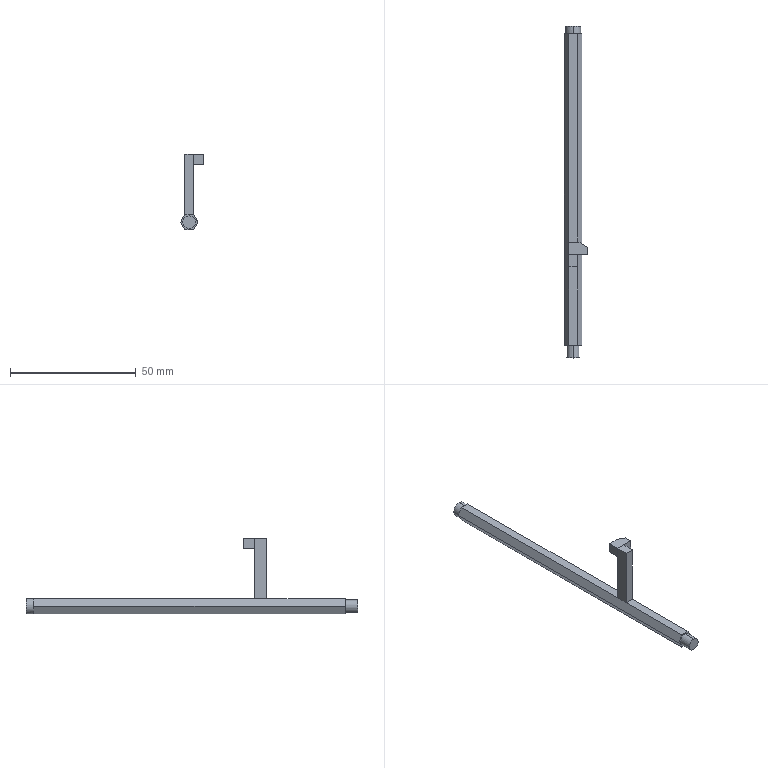Part | SolidWorks | features ICE 6, Cut 3, BaseBody 1, Chamfer 1 | 2 solids | 33 faces | box 9.182 x 132 x 30 mm | volume 4582 mm3 | plane 29 | cylinder 4 | commonest cylinder face diameters 5 x2 6 x2
STEP:
#1=CARTESIAN_POINT('',(-126.829,300.,155.684));
#2=VERTEX_POINT('',#1);
#3=CARTESIAN_POINT('',(-126.829,300.,149.684));
#4=VERTEX_POINT('',#3);
#5=CARTESIAN_POINT('',(-126.829,300.,152.684));
#6=DIRECTION('',(0.,1.,0.));
#7=DIRECTION('',(0.,0.,1.));
#8=AXIS2_PLACEMENT_3D('',#5,#6,#7);
#9=CIRCLE('',#8,3.);
#10=EDGE_CURVE('',#2,#4,#9,.T.);
#11=ORIENTED_EDGE('',*,*,#10,.F.);
#12=CARTESIAN_POINT('',(-126.829,297.,155.684));
#13=VERTEX_POINT('',#12);
#14=CARTESIAN_POINT('',(-126.829,302.,155.684));
#15=DIRECTION('',(0.,-1.,0.));
#16=VECTOR('',#15,1000.);
#17=LINE('',#14,#16);
#18=EDGE_CURVE('',#2,#13,#17,.T.);
#19=ORIENTED_EDGE('',*,*,#18,.T.);
#20=CARTESIAN_POINT('',(-124.231,297.,154.184));
#21=VERTEX_POINT('',#20);
#22=CARTESIAN_POINT('',(-126.829,297.,152.684));
#23=DIRECTION('',(0.,1.,0.));
#24=DIRECTION('',(1.,0.,0.));
#25=AXIS2_PLACEMENT_3D('',#22,#23,#24);
#26=CIRCLE('',#25,3.);
#27=EDGE_CURVE('',#13,#21,#26,.T.);
#28=ORIENTED_EDGE('',*,*,#27,.T.);
#29=CARTESIAN_POINT('',(-124.231,297.,151.184));
#30=VERTEX_POINT('',#29);
#31=CARTESIAN_POINT('',(-126.829,297.,152.684));
#32=DIRECTION('',(0.,1.,0.));
#33=DIRECTION('',(1.,0.,0.));
#34=AXIS2_PLACEMENT_3D('',#31,#32,#33);
#35=CIRCLE('',#34,3.);
#36=EDGE_CURVE('',#21,#30,#35,.T.);
#37=ORIENTED_EDGE('',*,*,#36,.T.);
#38=CARTESIAN_POINT('',(-126.829,297.,149.684));
#39=VERTEX_POINT('',#38);
#40=CARTESIAN_POINT('',(-126.829,297.,152.684));
#41=DIRECTION('',(0.,1.,0.));
#42=DIRECTION('',(1.,0.,0.));
#43=AXIS2_PLACEMENT_3D('',#40,#41,#42);
#44=CIRCLE('',#43,3.);
#45=EDGE_CURVE('',#30,#39,#44,.T.);
#46=ORIENTED_EDGE('',*,*,#45,.T.);
#47=CARTESIAN_POINT('',(-126.829,302.,149.684));
#48=DIRECTION('',(0.,-1.,0.));
#49=VECTOR('',#48,1000.);
#50=LINE('',#47,#49);
#51=EDGE_CURVE('',#4,#39,#50,.T.);
#52=ORIENTED_EDGE('',*,*,#51,.F.);
#53=EDGE_LOOP('',(#11,#19,#28,#37,#46,#52));
#54=FACE_OUTER_BOUND('',#53,.T.);
#55=CARTESIAN_POINT('',(-126.829,302.,152.684));
#56=DIRECTION('',(0.,-1.,0.));
#57=DIRECTION('',(0.,0.,-1.));
#58=AXIS2_PLACEMENT_3D('',#55,#56,#57);
#59=CYLINDRICAL_SURFACE('',#58,3.);
#60=ADVANCED_FACE('',(#54),#59,.T.);
#61=CARTESIAN_POINT('',(-126.829,168.,150.184));
#62=VERTEX_POINT('',#61);
#63=CARTESIAN_POINT('',(-126.829,168.,155.184));
#64=VERTEX_POINT('',#63);
#65=CARTESIAN_POINT('',(-126.829,168.,152.684));
#66=DIRECTION('',(0.,-1.,0.));
#67=DIRECTION('',(1.,0.,0.));
#68=AXIS2_PLACEMENT_3D('',#65,#66,#67);
#69=CIRCLE('',#68,2.5);
#70=EDGE_CURVE('',#62,#64,#69,.T.);
#71=ORIENTED_EDGE('',*,*,#70,.F.);
#72=CARTESIAN_POINT('',(-126.829,173.,150.184));
#73=VERTEX_POINT('',#72);
#74=CARTESIAN_POINT('',(-126.829,168.,150.184));
#75=DIRECTION('',(0.,1.,0.));
#76=VECTOR('',#75,1000.);
#77=LINE('',#74,#76);
#78=EDGE_CURVE('',#62,#73,#77,.T.);
#79=ORIENTED_EDGE('',*,*,#78,.T.);
#80=CARTESIAN_POINT('',(-126.829,173.,155.184));
#81=VERTEX_POINT('',#80);
#82=CARTESIAN_POINT('',(-126.829,173.,152.684));
#83=DIRECTION('',(0.,-1.,0.));
#84=DIRECTION('',(1.,0.,0.));
#85=AXIS2_PLACEMENT_3D('',#82,#83,#84);
#86=CIRCLE('',#85,2.5);
#87=EDGE_CURVE('',#73,#81,#86,.T.);
#88=ORIENTED_EDGE('',*,*,#87,.T.);
#89=CARTESIAN_POINT('',(-126.829,168.,155.184));
#90=DIRECTION('',(0.,1.,0.));
#91=VECTOR('',#90,1000.);
#92=LINE('',#89,#91);
#93=EDGE_CURVE('',#64,#81,#92,.T.);
#94=ORIENTED_EDGE('',*,*,#93,.F.);
#95=EDGE_LOOP('',(#71,#79,#88,#94));
#96=FACE_OUTER_BOUND('',#95,.T.);
#97=CARTESIAN_POINT('',(-126.829,168.,152.684));
#98=DIRECTION('',(0.,1.,0.));
#99=DIRECTION('',(0.,0.,1.));
#100=AXIS2_PLACEMENT_3D('',#97,#98,#99);
#101=CYLINDRICAL_SURFACE('',#100,2.5);
#102=ADVANCED_FACE('',(#96),#101,.T.);
#103=CARTESIAN_POINT('',(-128.561,209.118,179.684));
#104=VERTEX_POINT('',#103);
#105=CARTESIAN_POINT('',(-128.561,204.238,179.684));
#106=VERTEX_POINT('',#105);
#107=CARTESIAN_POINT('',(-128.561,217.498,179.684));
#108=DIRECTION('',(0.,-1.,0.));
#109=VECTOR('',#108,1000.);
#110=LINE('',#107,#109);
#111=EDGE_CURVE('',#104,#106,#110,.T.);
#112=ORIENTED_EDGE('',*,*,#111,.F.);
#113=CARTESIAN_POINT('',(-128.561,209.118,155.684));
#114=VERTEX_POINT('',#113);
#115=CARTESIAN_POINT('',(-128.561,209.118,155.684));
#116=DIRECTION('',(0.,0.,1.));
#117=VECTOR('',#116,1000.);
#118=LINE('',#115,#117);
#119=EDGE_CURVE('',#114,#104,#118,.T.);
#120=ORIENTED_EDGE('',*,*,#119,.F.);
#121=CARTESIAN_POINT('',(-128.561,204.238,155.684));
#122=VERTEX_POINT('',#121);
#123=CARTESIAN_POINT('',(-128.561,306.,155.684));
#124=DIRECTION('',(0.,-1.,0.));
#125=VECTOR('',#124,1000.);
#126=LINE('',#123,#125);
#127=EDGE_CURVE('',#114,#122,#126,.T.);
#128=ORIENTED_EDGE('',*,*,#127,.T.);
#129=CARTESIAN_POINT('',(-128.561,204.238,179.684));
#130=DIRECTION('',(0.,0.,1.));
#131=VECTOR('',#130,1000.);
#132=LINE('',#129,#131);
#133=EDGE_CURVE('',#122,#106,#132,.T.);
#134=ORIENTED_EDGE('',*,*,#133,.T.);
#135=EDGE_LOOP('',(#112,#120,#128,#134));
#136=FACE_OUTER_BOUND('',#135,.T.);
#137=CARTESIAN_POINT('',(-128.561,214.621,195.684));
#138=DIRECTION('',(1.,0.,0.));
#139=DIRECTION('',(0.,0.,-1.));
#140=AXIS2_PLACEMENT_3D('',#137,#138,#139);
#141=PLANE('',#140);
#142=ADVANCED_FACE('',(#136),#141,.F.);
#143=CARTESIAN_POINT('',(-125.096,209.118,179.684));
#144=VERTEX_POINT('',#143);
#145=CARTESIAN_POINT('',(5.,209.118,179.684));
#146=DIRECTION('',(1.,0.,0.));
#147=VECTOR('',#146,1000.);
#148=LINE('',#145,#147);
#149=EDGE_CURVE('',#104,#144,#148,.T.);
#150=ORIENTED_EDGE('',*,*,#149,.F.);
#151=ORIENTED_EDGE('',*,*,#111,.T.);
#152=CARTESIAN_POINT('',(-125.096,204.238,179.684));
#153=VERTEX_POINT('',#152);
#154=CARTESIAN_POINT('',(-125.096,204.238,179.684));
#155=DIRECTION('',(-1.,0.,0.));
#156=VECTOR('',#155,1000.);
#157=LINE('',#154,#156);
#158=EDGE_CURVE('',#153,#106,#157,.T.);
#159=ORIENTED_EDGE('',*,*,#158,.F.);
#160=CARTESIAN_POINT('',(-125.096,207.238,179.684));
#161=DIRECTION('',(0.,1.,0.));
#162=VECTOR('',#161,1000.);
#163=LINE('',#160,#162);
#164=EDGE_CURVE('',#153,#144,#163,.T.);
#165=ORIENTED_EDGE('',*,*,#164,.T.);
#166=EDGE_LOOP('',(#150,#151,#159,#165));
#167=FACE_OUTER_BOUND('',#166,.T.);
#168=CARTESIAN_POINT('',(5.,0.,179.684));
#169=DIRECTION('',(0.,0.,1.));
#170=DIRECTION('',(1.,0.,0.));
#171=AXIS2_PLACEMENT_3D('',#168,#169,#170);
#172=PLANE('',#171);
#173=ADVANCED_FACE('',(#167),#172,.T.);
#174=ORIENTED_EDGE('',*,*,#45,.F.);
#175=CARTESIAN_POINT('',(-125.097,297.,149.684));
#176=VERTEX_POINT('',#175);
#177=CARTESIAN_POINT('',(-123.365,297.,152.684));
#178=DIRECTION('',(-0.5,0.,-0.866));
#179=VECTOR('',#178,1000.);
#180=LINE('',#177,#179);
#181=EDGE_CURVE('',#30,#176,#180,.T.);
#182=ORIENTED_EDGE('',*,*,#181,.T.);
#183=CARTESIAN_POINT('',(-125.097,297.,149.684));
#184=DIRECTION('',(-1.,0.,0.));
#185=VECTOR('',#184,1000.);
#186=LINE('',#183,#185);
#187=EDGE_CURVE('',#176,#39,#186,.T.);
#188=ORIENTED_EDGE('',*,*,#187,.T.);
#189=EDGE_LOOP('',(#174,#182,#188));
#190=FACE_OUTER_BOUND('',#189,.T.);
#191=CARTESIAN_POINT('',(-195.,297.,35.));
#192=DIRECTION('',(0.,1.,0.));
#193=DIRECTION('',(0.,0.,-1.));
#194=AXIS2_PLACEMENT_3D('',#191,#192,#193);
#195=PLANE('',#194);
#196=ADVANCED_FACE('',(#190),#195,.T.);
#197=CARTESIAN_POINT('',(-129.427,297.,151.184));
#198=VERTEX_POINT('',#197);
#199=CARTESIAN_POINT('',(-126.829,297.,152.684));
#200=DIRECTION('',(0.,1.,0.));
#201=DIRECTION('',(1.,0.,0.));
#202=AXIS2_PLACEMENT_3D('',#199,#200,#201);
#203=CIRCLE('',#202,3.);
#204=EDGE_CURVE('',#39,#198,#203,.T.);
#205=ORIENTED_EDGE('',*,*,#204,.F.);
#206=CARTESIAN_POINT('',(-128.561,297.,149.684));
#207=VERTEX_POINT('',#206);
#208=CARTESIAN_POINT('',(-125.097,297.,149.684));
#209=DIRECTION('',(-1.,0.,0.));
#210=VECTOR('',#209,1000.);
#211=LINE('',#208,#210);
#212=EDGE_CURVE('',#39,#207,#211,.T.);
#213=ORIENTED_EDGE('',*,*,#212,.T.);
#214=CARTESIAN_POINT('',(-128.561,297.,149.684));
#215=DIRECTION('',(-0.5,0.,0.866));
#216=VECTOR('',#215,1000.);
#217=LINE('',#214,#216);
#218=EDGE_CURVE('',#207,#198,#217,.T.);
#219=ORIENTED_EDGE('',*,*,#218,.T.);
#220=EDGE_LOOP('',(#205,#213,#219));
#221=FACE_OUTER_BOUND('',#220,.T.);
#222=CARTESIAN_POINT('',(-195.,297.,35.));
#223=DIRECTION('',(0.,1.,0.));
#224=DIRECTION('',(0.,0.,-1.));
#225=AXIS2_PLACEMENT_3D('',#222,#223,#224);
#226=PLANE('',#225);
#227=ADVANCED_FACE('',(#221),#226,.T.);
#228=CARTESIAN_POINT('',(-129.427,297.,154.184));
#229=VERTEX_POINT('',#228);
#230=CARTESIAN_POINT('',(-126.829,297.,152.684));
#231=DIRECTION('',(0.,1.,0.));
#232=DIRECTION('',(1.,0.,0.));
#233=AXIS2_PLACEMENT_3D('',#230,#231,#232);
#234=CIRCLE('',#233,3.);
#235=EDGE_CURVE('',#198,#229,#234,.T.);
#236=ORIENTED_EDGE('',*,*,#235,.F.);
#237=CARTESIAN_POINT('',(-130.293,297.,152.684));
#238=VERTEX_POINT('',#237);
#239=CARTESIAN_POINT('',(-128.561,297.,149.684));
#240=DIRECTION('',(-0.5,0.,0.866));
#241=VECTOR('',#240,1000.);
#242=LINE('',#239,#241);
#243=EDGE_CURVE('',#198,#238,#242,.T.);
#244=ORIENTED_EDGE('',*,*,#243,.T.);
#245=CARTESIAN_POINT('',(-130.293,297.,152.684));
#246=DIRECTION('',(0.5,0.,0.866));
#247=VECTOR('',#246,1000.);
#248=LINE('',#245,#247);
#249=EDGE_CURVE('',#238,#229,#248,.T.);
#250=ORIENTED_EDGE('',*,*,#249,.T.);
#251=EDGE_LOOP('',(#236,#244,#250));
#252=FACE_OUTER_BOUND('',#251,.T.);
#253=CARTESIAN_POINT('',(-195.,297.,35.));
#254=DIRECTION('',(0.,1.,0.));
#255=DIRECTION('',(0.,0.,-1.));
#256=AXIS2_PLACEMENT_3D('',#253,#254,#255);
#257=PLANE('',#256);
#258=ADVANCED_FACE('',(#252),#257,.T.);
#259=CARTESIAN_POINT('',(-126.829,297.,152.684));
#260=DIRECTION('',(0.,1.,0.));
#261=DIRECTION('',(1.,0.,0.));
#262=AXIS2_PLACEMENT_3D('',#259,#260,#261);
#263=CIRCLE('',#262,3.);
#264=EDGE_CURVE('',#229,#13,#263,.T.);
#265=ORIENTED_EDGE('',*,*,#264,.F.);
#266=CARTESIAN_POINT('',(-128.561,297.,155.684));
#267=VERTEX_POINT('',#266);
#268=CARTESIAN_POINT('',(-130.293,297.,152.684));
#269=DIRECTION('',(0.5,0.,0.866));
#270=VECTOR('',#269,1000.);
#271=LINE('',#268,#270);
#272=EDGE_CURVE('',#229,#267,#271,.T.);
#273=ORIENTED_EDGE('',*,*,#272,.T.);
#274=CARTESIAN_POINT('',(-128.561,297.,155.684));
#275=DIRECTION('',(1.,0.,0.));
#276=VECTOR('',#275,1000.);
#277=LINE('',#274,#276);
#278=EDGE_CURVE('',#267,#13,#277,.T.);
#279=ORIENTED_EDGE('',*,*,#278,.T.);
#280=EDGE_LOOP('',(#265,#273,#279));
#281=FACE_OUTER_BOUND('',#280,.T.);
#282=CARTESIAN_POINT('',(-195.,297.,35.));
#283=DIRECTION('',(0.,1.,0.));
#284=DIRECTION('',(0.,0.,-1.));
#285=AXIS2_PLACEMENT_3D('',#282,#283,#284);
#286=PLANE('',#285);
#287=ADVANCED_FACE('',(#281),#286,.T.);
#288=ORIENTED_EDGE('',*,*,#27,.F.);
#289=CARTESIAN_POINT('',(-125.097,297.,155.684));
#290=VERTEX_POINT('',#289);
#291=CARTESIAN_POINT('',(-128.561,297.,155.684));
#292=DIRECTION('',(1.,0.,0.));
#293=VECTOR('',#292,1000.);
#294=LINE('',#291,#293);
#295=EDGE_CURVE('',#13,#290,#294,.T.);
#296=ORIENTED_EDGE('',*,*,#295,.T.);
#297=CARTESIAN_POINT('',(-125.097,297.,155.684));
#298=DIRECTION('',(0.5,0.,-0.866));
#299=VECTOR('',#298,1000.);
#300=LINE('',#297,#299);
#301=EDGE_CURVE('',#290,#21,#300,.T.);
#302=ORIENTED_EDGE('',*,*,#301,.T.);
#303=EDGE_LOOP('',(#288,#296,#302));
#304=FACE_OUTER_BOUND('',#303,.T.);
#305=CARTESIAN_POINT('',(-195.,297.,35.));
#306=DIRECTION('',(0.,1.,0.));
#307=DIRECTION('',(0.,0.,-1.));
#308=AXIS2_PLACEMENT_3D('',#305,#306,#307);
#309=PLANE('',#308);
#310=ADVANCED_FACE('',(#304),#309,.T.);
#311=CARTESIAN_POINT('',(-128.561,214.621,155.684));
#312=DIRECTION('',(0.,-1.,0.));
#313=VECTOR('',#312,1000.);
#314=LINE('',#311,#313);
#315=EDGE_CURVE('',#267,#114,#314,.T.);
#316=ORIENTED_EDGE('',*,*,#315,.T.);
#317=CARTESIAN_POINT('',(-125.096,209.118,155.684));
#318=VERTEX_POINT('',#317);
#319=CARTESIAN_POINT('',(-104.061,209.118,155.684));
#320=DIRECTION('',(-1.,0.,0.));
#321=VECTOR('',#320,1000.);
#322=LINE('',#319,#321);
#323=EDGE_CURVE('',#318,#114,#322,.T.);
#324=ORIENTED_EDGE('',*,*,#323,.F.);
#325=CARTESIAN_POINT('',(-125.096,212.118,155.684));
#326=VERTEX_POINT('',#325);
#327=CARTESIAN_POINT('',(-125.096,0.,155.684));
#328=DIRECTION('',(0.,1.,0.));
#329=VECTOR('',#328,1000.);
#330=LINE('',#327,#329);
#331=EDGE_CURVE('',#318,#326,#330,.T.);
#332=ORIENTED_EDGE('',*,*,#331,.T.);
#333=CARTESIAN_POINT('',(-125.097,212.118,155.684));
#334=VERTEX_POINT('',#333);
#335=CARTESIAN_POINT('',(-115.561,212.118,155.684));
#336=DIRECTION('',(1.,0.,0.));
#337=VECTOR('',#336,1000.);
#338=LINE('',#335,#337);
#339=EDGE_CURVE('',#334,#326,#338,.T.);
#340=ORIENTED_EDGE('',*,*,#339,.F.);
#341=CARTESIAN_POINT('',(-125.097,306.,155.684));
#342=DIRECTION('',(0.,-1.,0.));
#343=VECTOR('',#342,1000.);
#344=LINE('',#341,#343);
#345=EDGE_CURVE('',#290,#334,#344,.T.);
#346=ORIENTED_EDGE('',*,*,#345,.F.);
#347=ORIENTED_EDGE('',*,*,#295,.F.);
#348=ORIENTED_EDGE('',*,*,#278,.F.);
#349=EDGE_LOOP('',(#316,#324,#332,#340,#346,#347,#348));
#350=FACE_OUTER_BOUND('',#349,.T.);
#351=CARTESIAN_POINT('',(-128.561,306.,155.684));
#352=DIRECTION('',(0.,0.,-1.));
#353=DIRECTION('',(-1.,0.,0.));
#354=AXIS2_PLACEMENT_3D('',#351,#352,#353);
#355=PLANE('',#354);
#356=ADVANCED_FACE('',(#350),#355,.F.);
#357=CARTESIAN_POINT('',(-125.097,204.238,155.684));
#358=VERTEX_POINT('',#357);
#359=CARTESIAN_POINT('',(-125.097,173.,155.684));
#360=VERTEX_POINT('',#359);
#361=CARTESIAN_POINT('',(-125.097,306.,155.684));
#362=DIRECTION('',(0.,-1.,0.));
#363=VECTOR('',#362,1000.);
#364=LINE('',#361,#363);
#365=EDGE_CURVE('',#358,#360,#364,.T.);
#366=ORIENTED_EDGE('',*,*,#365,.F.);
#367=CARTESIAN_POINT('',(-125.096,204.238,155.684));
#368=DIRECTION('',(-1.,0.,0.));
#369=VECTOR('',#368,1000.);
#370=LINE('',#367,#369);
#371=EDGE_CURVE('',#358,#122,#370,.T.);
#372=ORIENTED_EDGE('',*,*,#371,.T.);
#373=CARTESIAN_POINT('',(-128.561,173.,155.684));
#374=VERTEX_POINT('',#373);
#375=CARTESIAN_POINT('',(-128.561,306.,155.684));
#376=DIRECTION('',(0.,-1.,0.));
#377=VECTOR('',#376,1000.);
#378=LINE('',#375,#377);
#379=EDGE_CURVE('',#122,#374,#378,.T.);
#380=ORIENTED_EDGE('',*,*,#379,.T.);
#381=CARTESIAN_POINT('',(-128.561,173.,155.684));
#382=DIRECTION('',(1.,0.,0.));
#383=VECTOR('',#382,1000.);
#384=LINE('',#381,#383);
#385=EDGE_CURVE('',#374,#360,#384,.T.);
#386=ORIENTED_EDGE('',*,*,#385,.T.);
#387=EDGE_LOOP('',(#366,#372,#380,#386));
#388=FACE_OUTER_BOUND('',#387,.T.);
#389=CARTESIAN_POINT('',(-128.561,306.,155.684));
#390=DIRECTION('',(0.,0.,-1.));
#391=DIRECTION('',(-1.,0.,0.));
#392=AXIS2_PLACEMENT_3D('',#389,#390,#391);
#393=PLANE('',#392);
#394=ADVANCED_FACE('',(#388),#393,.F.);
#395=ORIENTED_EDGE('',*,*,#345,.T.);
#396=CARTESIAN_POINT('',(-125.096,212.118,155.682));
#397=VERTEX_POINT('',#396);
#398=CARTESIAN_POINT('',(-125.097,212.118,155.684));
#399=DIRECTION('',(0.5,0.,-0.866));
#400=VECTOR('',#399,1000.);
#401=LINE('',#398,#400);
#402=EDGE_CURVE('',#334,#397,#401,.T.);
#403=ORIENTED_EDGE('',*,*,#402,.T.);
#404=CARTESIAN_POINT('',(-125.096,204.238,155.682));
#405=VERTEX_POINT('',#404);
#406=CARTESIAN_POINT('',(-125.096,306.,155.682));
#407=DIRECTION('',(0.,-1.,0.));
#408=VECTOR('',#407,1000.);
#409=LINE('',#406,#408);
#410=EDGE_CURVE('',#397,#405,#409,.T.);
#411=ORIENTED_EDGE('',*,*,#410,.T.);
#412=CARTESIAN_POINT('',(-125.097,204.238,155.684));
#413=DIRECTION('',(-0.5,0.,0.866));
#414=VECTOR('',#413,1000.);
#415=LINE('',#412,#414);
#416=EDGE_CURVE('',#405,#358,#415,.T.);
#417=ORIENTED_EDGE('',*,*,#416,.T.);
#418=ORIENTED_EDGE('',*,*,#365,.T.);
#419=CARTESIAN_POINT('',(-123.365,173.,152.684));
#420=VERTEX_POINT('',#419);
#421=CARTESIAN_POINT('',(-125.097,173.,155.684));
#422=DIRECTION('',(0.5,0.,-0.866));
#423=VECTOR('',#422,1000.);
#424=LINE('',#421,#423);
#425=EDGE_CURVE('',#360,#420,#424,.T.);
#426=ORIENTED_EDGE('',*,*,#425,.T.);
#427=CARTESIAN_POINT('',(-123.365,297.,152.684));
#428=VERTEX_POINT('',#427);
#429=CARTESIAN_POINT('',(-123.365,306.,152.684));
#430=DIRECTION('',(0.,-1.,0.));
#431=VECTOR('',#430,1000.);
#432=LINE('',#429,#431);
#433=EDGE_CURVE('',#428,#420,#432,.T.);
#434=ORIENTED_EDGE('',*,*,#433,.F.);
#435=CARTESIAN_POINT('',(-125.097,297.,155.684));
#436=DIRECTION('',(0.5,0.,-0.866));
#437=VECTOR('',#436,1000.);
#438=LINE('',#435,#437);
#439=EDGE_CURVE('',#21,#428,#438,.T.);
#440=ORIENTED_EDGE('',*,*,#439,.F.);
#441=ORIENTED_EDGE('',*,*,#301,.F.);
#442=EDGE_LOOP('',(#395,#403,#411,#417,#418,#426,#434,#440,#441));
#443=FACE_OUTER_BOUND('',#442,.T.);
#444=CARTESIAN_POINT('',(-125.097,306.,155.684));
#445=DIRECTION('',(-0.866,0.,-0.5));
#446=DIRECTION('',(-0.5,0.,0.866));
#447=AXIS2_PLACEMENT_3D('',#444,#445,#446);
#448=PLANE('',#447);
#449=ADVANCED_FACE('',(#443),#448,.F.);
#450=ORIENTED_EDGE('',*,*,#433,.T.);
#451=CARTESIAN_POINT('',(-125.097,173.,149.684));
#452=VERTEX_POINT('',#451);
#453=CARTESIAN_POINT('',(-123.365,173.,152.684));
#454=DIRECTION('',(-0.5,0.,-0.866));
#455=VECTOR('',#454,1000.);
#456=LINE('',#453,#455);
#457=EDGE_CURVE('',#420,#452,#456,.T.);
#458=ORIENTED_EDGE('',*,*,#457,.T.);
#459=CARTESIAN_POINT('',(-125.097,306.,149.684));
#460=DIRECTION('',(0.,-1.,0.));
#461=VECTOR('',#460,1000.);
#462=LINE('',#459,#461);
#463=EDGE_CURVE('',#176,#452,#462,.T.);
#464=ORIENTED_EDGE('',*,*,#463,.F.);
#465=ORIENTED_EDGE('',*,*,#181,.F.);
#466=CARTESIAN_POINT('',(-123.365,297.,152.684));
#467=DIRECTION('',(-0.5,0.,-0.866));
#468=VECTOR('',#467,1000.);
#469=LINE('',#466,#468);
#470=EDGE_CURVE('',#428,#30,#469,.T.);
#471=ORIENTED_EDGE('',*,*,#470,.F.);
#472=EDGE_LOOP('',(#450,#458,#464,#465,#471));
#473=FACE_OUTER_BOUND('',#472,.T.);
#474=CARTESIAN_POINT('',(-123.365,306.,152.684));
#475=DIRECTION('',(-0.866,0.,0.5));
#476=DIRECTION('',(0.5,0.,0.866));
#477=AXIS2_PLACEMENT_3D('',#474,#475,#476);
#478=PLANE('',#477);
#479=ADVANCED_FACE('',(#473),#478,.F.);
#480=ORIENTED_EDGE('',*,*,#463,.T.);
#481=CARTESIAN_POINT('',(-128.561,173.,149.684));
#482=VERTEX_POINT('',#481);
#483=CARTESIAN_POINT('',(-125.097,173.,149.684));
#484=DIRECTION('',(-1.,0.,0.));
#485=VECTOR('',#484,1000.);
#486=LINE('',#483,#485);
#487=EDGE_CURVE('',#452,#482,#486,.T.);
#488=ORIENTED_EDGE('',*,*,#487,.T.);
#489=CARTESIAN_POINT('',(-128.561,306.,149.684));
#490=DIRECTION('',(0.,-1.,0.));
#491=VECTOR('',#490,1000.);
#492=LINE('',#489,#491);
#493=EDGE_CURVE('',#207,#482,#492,.T.);
#494=ORIENTED_EDGE('',*,*,#493,.F.);
#495=ORIENTED_EDGE('',*,*,#212,.F.);
#496=ORIENTED_EDGE('',*,*,#187,.F.);
#497=EDGE_LOOP('',(#480,#488,#494,#495,#496));
#498=FACE_OUTER_BOUND('',#497,.T.);
#499=CARTESIAN_POINT('',(-125.097,306.,149.684));
#500=DIRECTION('',(0.,0.,1.));
#501=DIRECTION('',(1.,0.,0.));
#502=AXIS2_PLACEMENT_3D('',#499,#500,#501);
#503=PLANE('',#502);
#504=ADVANCED_FACE('',(#498),#503,.F.);
#505=ORIENTED_EDGE('',*,*,#493,.T.);
#506=CARTESIAN_POINT('',(-130.293,173.,152.684));
#507=VERTEX_POINT('',#506);
#508=CARTESIAN_POINT('',(-128.561,173.,149.684));
#509=DIRECTION('',(-0.5,0.,0.866));
#510=VECTOR('',#509,1000.);
#511=LINE('',#508,#510);
#512=EDGE_CURVE('',#482,#507,#511,.T.);
#513=ORIENTED_EDGE('',*,*,#512,.T.);
#514=CARTESIAN_POINT('',(-130.293,306.,152.684));
#515=DIRECTION('',(0.,-1.,0.));
#516=VECTOR('',#515,1000.);
#517=LINE('',#514,#516);
#518=EDGE_CURVE('',#238,#507,#517,.T.);
#519=ORIENTED_EDGE('',*,*,#518,.F.);
#520=ORIENTED_EDGE('',*,*,#243,.F.);
#521=ORIENTED_EDGE('',*,*,#218,.F.);
#522=EDGE_LOOP('',(#505,#513,#519,#520,#521));
#523=FACE_OUTER_BOUND('',#522,.T.);
#524=CARTESIAN_POINT('',(-128.561,306.,149.684));
#525=DIRECTION('',(0.866,0.,0.5));
#526=DIRECTION('',(0.5,0.,-0.866));
#527=AXIS2_PLACEMENT_3D('',#524,#525,#526);
#528=PLANE('',#527);
#529=ADVANCED_FACE('',(#523),#528,.F.);
#530=ORIENTED_EDGE('',*,*,#518,.T.);
#531=CARTESIAN_POINT('',(-130.293,173.,152.684));
#532=DIRECTION('',(0.5,0.,0.866));
#533=VECTOR('',#532,1000.);
#534=LINE('',#531,#533);
#535=EDGE_CURVE('',#507,#374,#534,.T.);
#536=ORIENTED_EDGE('',*,*,#535,.T.);
#537=ORIENTED_EDGE('',*,*,#379,.F.);
#538=ORIENTED_EDGE('',*,*,#127,.F.);
#539=ORIENTED_EDGE('',*,*,#315,.F.);
#540=ORIENTED_EDGE('',*,*,#272,.F.);
#541=ORIENTED_EDGE('',*,*,#249,.F.);
#542=EDGE_LOOP('',(#530,#536,#537,#538,#539,#540,#541));
#543=FACE_OUTER_BOUND('',#542,.T.);
#544=CARTESIAN_POINT('',(-130.293,306.,152.684));
#545=DIRECTION('',(0.866,0.,-0.5));
#546=DIRECTION('',(-0.5,0.,-0.866));
#547=AXIS2_PLACEMENT_3D('',#544,#545,#546);
#548=PLANE('',#547);
#549=ADVANCED_FACE('',(#543),#548,.F.);
#550=ORIENTED_EDGE('',*,*,#36,.F.);
#551=ORIENTED_EDGE('',*,*,#439,.T.);
#552=ORIENTED_EDGE('',*,*,#470,.T.);
#553=EDGE_LOOP('',(#550,#551,#552));
#554=FACE_OUTER_BOUND('',#553,.T.);
#555=CARTESIAN_POINT('',(-195.,297.,35.));
#556=DIRECTION('',(0.,1.,0.));
#557=DIRECTION('',(0.,0.,-1.));
#558=AXIS2_PLACEMENT_3D('',#555,#556,#557);
#559=PLANE('',#558);
#560=ADVANCED_FACE('',(#554),#559,.T.);
#561=CARTESIAN_POINT('',(-126.829,173.,152.684));
#562=DIRECTION('',(0.,-1.,0.));
#563=DIRECTION('',(1.,0.,0.));
#564=AXIS2_PLACEMENT_3D('',#561,#562,#563);
#565=CIRCLE('',#564,2.5);
#566=EDGE_CURVE('',#81,#73,#565,.T.);
#567=ORIENTED_EDGE('',*,*,#566,.F.);
#568=ORIENTED_EDGE('',*,*,#87,.F.);
#569=EDGE_LOOP('',(#567,#568));
#570=FACE_BOUND('',#569,.T.);
#571=ORIENTED_EDGE('',*,*,#385,.F.);
#572=ORIENTED_EDGE('',*,*,#535,.F.);
#573=ORIENTED_EDGE('',*,*,#512,.F.);
#574=ORIENTED_EDGE('',*,*,#487,.F.);
#575=ORIENTED_EDGE('',*,*,#457,.F.);
#576=ORIENTED_EDGE('',*,*,#425,.F.);
#577=EDGE_LOOP('',(#571,#572,#573,#574,#575,#576));
#578=FACE_OUTER_BOUND('',#577,.T.);
#579=CARTESIAN_POINT('',(5.,173.,35.));
#580=DIRECTION('',(0.,1.,0.));
#581=DIRECTION('',(0.,0.,1.));
#582=AXIS2_PLACEMENT_3D('',#579,#580,#581);
#583=PLANE('',#582);
#584=ADVANCED_FACE('',(#570,#578),#583,.F.);
#585=ORIENTED_EDGE('',*,*,#78,.F.);
#586=CARTESIAN_POINT('',(-126.829,168.,152.684));
#587=DIRECTION('',(0.,-1.,0.));
#588=DIRECTION('',(1.,0.,0.));
#589=AXIS2_PLACEMENT_3D('',#586,#587,#588);
#590=CIRCLE('',#589,2.5);
#591=EDGE_CURVE('',#64,#62,#590,.T.);
#592=ORIENTED_EDGE('',*,*,#591,.F.);
#593=ORIENTED_EDGE('',*,*,#93,.T.);
#594=ORIENTED_EDGE('',*,*,#566,.T.);
#595=EDGE_LOOP('',(#585,#592,#593,#594));
#596=FACE_OUTER_BOUND('',#595,.T.);
#597=CARTESIAN_POINT('',(-126.829,168.,152.684));
#598=DIRECTION('',(0.,1.,0.));
#599=DIRECTION('',(0.,0.,1.));
#600=AXIS2_PLACEMENT_3D('',#597,#598,#599);
#601=CYLINDRICAL_SURFACE('',#600,2.5);
#602=ADVANCED_FACE('',(#596),#601,.T.);
#603=ORIENTED_EDGE('',*,*,#591,.T.);
#604=ORIENTED_EDGE('',*,*,#70,.T.);
#605=EDGE_LOOP('',(#603,#604));
#606=FACE_OUTER_BOUND('',#605,.T.);
#607=CARTESIAN_POINT('',(-126.829,168.,152.684));
#608=DIRECTION('',(0.,-1.,0.));
#609=DIRECTION('',(0.,0.,-1.));
#610=AXIS2_PLACEMENT_3D('',#607,#608,#609);
#611=PLANE('',#610);
#612=ADVANCED_FACE('',(#606),#611,.T.);
#613=ORIENTED_EDGE('',*,*,#18,.F.);
#614=CARTESIAN_POINT('',(-126.829,300.,152.684));
#615=DIRECTION('',(0.,1.,0.));
#616=DIRECTION('',(0.,0.,1.));
#617=AXIS2_PLACEMENT_3D('',#614,#615,#616);
#618=CIRCLE('',#617,3.);
#619=EDGE_CURVE('',#4,#2,#618,.T.);
#620=ORIENTED_EDGE('',*,*,#619,.F.);
#621=ORIENTED_EDGE('',*,*,#51,.T.);
#622=ORIENTED_EDGE('',*,*,#204,.T.);
#623=ORIENTED_EDGE('',*,*,#235,.T.);
#624=ORIENTED_EDGE('',*,*,#264,.T.);
#625=EDGE_LOOP('',(#613,#620,#621,#622,#623,#624));
#626=FACE_OUTER_BOUND('',#625,.T.);
#627=CARTESIAN_POINT('',(-126.829,302.,152.684));
#628=DIRECTION('',(0.,-1.,0.));
#629=DIRECTION('',(0.,0.,-1.));
#630=AXIS2_PLACEMENT_3D('',#627,#628,#629);
#631=CYLINDRICAL_SURFACE('',#630,3.);
#632=ADVANCED_FACE('',(#626),#631,.T.);
#633=ORIENTED_EDGE('',*,*,#619,.T.);
#634=ORIENTED_EDGE('',*,*,#10,.T.);
#635=EDGE_LOOP('',(#633,#634));
#636=FACE_OUTER_BOUND('',#635,.T.);
#637=CARTESIAN_POINT('',(-200.,300.,0.));
#638=DIRECTION('',(0.,1.,0.));
#639=DIRECTION('',(0.,0.,-1.));
#640=AXIS2_PLACEMENT_3D('',#637,#638,#639);
#641=PLANE('',#640);
#642=ADVANCED_FACE('',(#636),#641,.T.);
#643=ORIENTED_EDGE('',*,*,#402,.F.);
#644=ORIENTED_EDGE('',*,*,#339,.T.);
#645=CARTESIAN_POINT('',(-125.096,212.118,155.184));
#646=DIRECTION('',(0.,0.,1.));
#647=VECTOR('',#646,1000.);
#648=LINE('',#645,#647);
#649=EDGE_CURVE('',#397,#326,#648,.T.);
#650=ORIENTED_EDGE('',*,*,#649,.F.);
#651=EDGE_LOOP('',(#643,#644,#650));
#652=FACE_OUTER_BOUND('',#651,.T.);
#653=CARTESIAN_POINT('',(-115.561,212.118,173.));
#654=DIRECTION('',(0.,-1.,0.));
#655=DIRECTION('',(0.,0.,-1.));
#656=AXIS2_PLACEMENT_3D('',#653,#654,#655);
#657=PLANE('',#656);
#658=ADVANCED_FACE('',(#652),#657,.F.);
#659=ORIENTED_EDGE('',*,*,#133,.F.);
#660=ORIENTED_EDGE('',*,*,#371,.F.);
#661=ORIENTED_EDGE('',*,*,#416,.F.);
#662=CARTESIAN_POINT('',(-125.096,204.238,179.684));
#663=DIRECTION('',(0.,0.,1.));
#664=VECTOR('',#663,1000.);
#665=LINE('',#662,#664);
#666=EDGE_CURVE('',#405,#153,#665,.T.);
#667=ORIENTED_EDGE('',*,*,#666,.T.);
#668=ORIENTED_EDGE('',*,*,#158,.T.);
#669=EDGE_LOOP('',(#659,#660,#661,#667,#668));
#670=FACE_OUTER_BOUND('',#669,.T.);
#671=CARTESIAN_POINT('',(-125.096,204.238,179.684));
#672=DIRECTION('',(0.,-1.,0.));
#673=DIRECTION('',(0.,0.,-1.));
#674=AXIS2_PLACEMENT_3D('',#671,#672,#673);
#675=PLANE('',#674);
#676=ADVANCED_FACE('',(#670),#675,.T.);
#677=ORIENTED_EDGE('',*,*,#331,.F.);
#678=CARTESIAN_POINT('',(-125.096,209.118,0.));
#679=DIRECTION('',(0.,0.,-1.));
#680=VECTOR('',#679,1000.);
#681=LINE('',#678,#680);
#682=EDGE_CURVE('',#144,#318,#681,.T.);
#683=ORIENTED_EDGE('',*,*,#682,.F.);
#684=ORIENTED_EDGE('',*,*,#164,.F.);
#685=ORIENTED_EDGE('',*,*,#666,.F.);
#686=ORIENTED_EDGE('',*,*,#410,.F.);
#687=ORIENTED_EDGE('',*,*,#649,.T.);
#688=EDGE_LOOP('',(#677,#683,#684,#685,#686,#687));
#689=FACE_OUTER_BOUND('',#688,.T.);
#690=CARTESIAN_POINT('',(-125.096,0.,0.));
#691=DIRECTION('',(1.,0.,0.));
#692=DIRECTION('',(0.,0.,-1.));
#693=AXIS2_PLACEMENT_3D('',#690,#691,#692);
#694=PLANE('',#693);
#695=ADVANCED_FACE('',(#689),#694,.T.);
#696=ORIENTED_EDGE('',*,*,#149,.T.);
#697=ORIENTED_EDGE('',*,*,#682,.T.);
#698=ORIENTED_EDGE('',*,*,#323,.T.);
#699=ORIENTED_EDGE('',*,*,#119,.T.);
#700=EDGE_LOOP('',(#696,#697,#698,#699));
#701=FACE_OUTER_BOUND('',#700,.T.);
#702=CARTESIAN_POINT('',(-104.061,209.118,155.684));
#703=DIRECTION('',(0.,-1.,0.));
#704=DIRECTION('',(0.,0.,-1.));
#705=AXIS2_PLACEMENT_3D('',#702,#703,#704);
#706=PLANE('',#705);
#707=ADVANCED_FACE('',(#701),#706,.F.);
#708=CLOSED_SHELL('',(#60,#102,#142,#173,#196,#227,#258,#287,#310,#356,#394,#449,#479,#504,#529,#549,#560,#584,#602,#612,#632,#642,#658,#676,#695,#707));
#709=MANIFOLD_SOLID_BREP('',#708);
#710=CARTESIAN_POINT('',(-124.111,213.718,175.678));
#711=VERTEX_POINT('',#710);
#712=CARTESIAN_POINT('',(-128.561,213.718,175.678));
#713=VERTEX_POINT('',#712);
#714=CARTESIAN_POINT('',(-128.561,213.718,175.678));
#715=DIRECTION('',(-1.,0.,0.));
#716=VECTOR('',#715,1000.);
#717=LINE('',#714,#716);
#718=EDGE_CURVE('',#711,#713,#717,.T.);
#719=ORIENTED_EDGE('',*,*,#718,.F.);
#720=CARTESIAN_POINT('',(-121.111,211.986,175.678));
#721=VERTEX_POINT('',#720);
#722=CARTESIAN_POINT('',(-122.869,213.001,175.678));
#723=DIRECTION('',(0.866,-0.5,0.));
#724=VECTOR('',#723,1000.);
#725=LINE('',#722,#724);
#726=EDGE_CURVE('',#711,#721,#725,.T.);
#727=ORIENTED_EDGE('',*,*,#726,.T.);
#728=CARTESIAN_POINT('',(-121.111,209.118,175.678));
#729=VERTEX_POINT('',#728);
#730=CARTESIAN_POINT('',(-121.111,211.718,175.678));
#731=DIRECTION('',(0.,1.,0.));
#732=VECTOR('',#731,1000.);
#733=LINE('',#730,#732);
#734=EDGE_CURVE('',#729,#721,#733,.T.);
#735=ORIENTED_EDGE('',*,*,#734,.F.);
#736=CARTESIAN_POINT('',(-128.561,209.118,175.678));
#737=VERTEX_POINT('',#736);
#738=CARTESIAN_POINT('',(-125.111,209.118,175.678));
#739=DIRECTION('',(-1.,0.,0.));
#740=VECTOR('',#739,1000.);
#741=LINE('',#738,#740);
#742=EDGE_CURVE('',#729,#737,#741,.T.);
#743=ORIENTED_EDGE('',*,*,#742,.T.);
#744=CARTESIAN_POINT('',(-128.561,209.118,175.678));
#745=DIRECTION('',(0.,-1.,0.));
#746=VECTOR('',#745,1000.);
#747=LINE('',#744,#746);
#748=EDGE_CURVE('',#713,#737,#747,.T.);
#749=ORIENTED_EDGE('',*,*,#748,.F.);
#750=EDGE_LOOP('',(#719,#727,#735,#743,#749));
#751=FACE_OUTER_BOUND('',#750,.T.);
#752=CARTESIAN_POINT('',(-125.111,209.118,175.678));
#753=DIRECTION('',(0.,0.,-1.));
#754=DIRECTION('',(-1.,0.,0.));
#755=AXIS2_PLACEMENT_3D('',#752,#753,#754);
#756=PLANE('',#755);
#757=ADVANCED_FACE('',(#751),#756,.T.);
#758=CARTESIAN_POINT('',(-121.111,211.986,179.684));
#759=VERTEX_POINT('',#758);
#760=CARTESIAN_POINT('',(-121.111,209.118,179.684));
#761=VERTEX_POINT('',#760);
#762=CARTESIAN_POINT('',(-121.111,211.718,179.684));
#763=DIRECTION('',(0.,-1.,0.));
#764=VECTOR('',#763,1000.);
#765=LINE('',#762,#764);
#766=EDGE_CURVE('',#759,#761,#765,.T.);
#767=ORIENTED_EDGE('',*,*,#766,.F.);
#768=CARTESIAN_POINT('',(-124.111,213.718,179.684));
#769=VERTEX_POINT('',#768);
#770=CARTESIAN_POINT('',(-122.869,213.001,179.684));
#771=DIRECTION('',(-0.866,0.5,0.));
#772=VECTOR('',#771,1000.);
#773=LINE('',#770,#772);
#774=EDGE_CURVE('',#759,#769,#773,.T.);
#775=ORIENTED_EDGE('',*,*,#774,.T.);
#776=CARTESIAN_POINT('',(-128.561,213.718,179.684));
#777=VERTEX_POINT('',#776);
#778=CARTESIAN_POINT('',(-128.561,213.718,179.684));
#779=DIRECTION('',(1.,0.,0.));
#780=VECTOR('',#779,1000.);
#781=LINE('',#778,#780);
#782=EDGE_CURVE('',#777,#769,#781,.T.);
#783=ORIENTED_EDGE('',*,*,#782,.F.);
#784=CARTESIAN_POINT('',(-128.561,209.118,179.684));
#785=VERTEX_POINT('',#784);
#786=CARTESIAN_POINT('',(-128.561,209.118,179.684));
#787=DIRECTION('',(0.,1.,0.));
#788=VECTOR('',#787,1000.);
#789=LINE('',#786,#788);
#790=EDGE_CURVE('',#785,#777,#789,.T.);
#791=ORIENTED_EDGE('',*,*,#790,.F.);
#792=CARTESIAN_POINT('',(-125.111,209.118,179.684));
#793=DIRECTION('',(-1.,0.,0.));
#794=VECTOR('',#793,1000.);
#795=LINE('',#792,#794);
#796=EDGE_CURVE('',#761,#785,#795,.T.);
#797=ORIENTED_EDGE('',*,*,#796,.F.);
#798=EDGE_LOOP('',(#767,#775,#783,#791,#797));
#799=FACE_OUTER_BOUND('',#798,.T.);
#800=CARTESIAN_POINT('',(-125.111,209.118,179.684));
#801=DIRECTION('',(0.,0.,1.));
#802=DIRECTION('',(1.,0.,0.));
#803=AXIS2_PLACEMENT_3D('',#800,#801,#802);
#804=PLANE('',#803);
#805=ADVANCED_FACE('',(#799),#804,.T.);
#806=CARTESIAN_POINT('',(-128.561,209.118,175.678));
#807=DIRECTION('',(0.,0.,1.));
#808=VECTOR('',#807,1000.);
#809=LINE('',#806,#808);
#810=EDGE_CURVE('',#737,#785,#809,.T.);
#811=ORIENTED_EDGE('',*,*,#810,.F.);
#812=ORIENTED_EDGE('',*,*,#742,.F.);
#813=CARTESIAN_POINT('',(-121.111,209.118,179.684));
#814=DIRECTION('',(0.,0.,-1.));
#815=VECTOR('',#814,1000.);
#816=LINE('',#813,#815);
#817=EDGE_CURVE('',#761,#729,#816,.T.);
#818=ORIENTED_EDGE('',*,*,#817,.F.);
#819=ORIENTED_EDGE('',*,*,#796,.T.);
#820=EDGE_LOOP('',(#811,#812,#818,#819));
#821=FACE_OUTER_BOUND('',#820,.T.);
#822=CARTESIAN_POINT('',(-125.111,209.118,175.678));
#823=DIRECTION('',(0.,-1.,0.));
#824=DIRECTION('',(0.,0.,-1.));
#825=AXIS2_PLACEMENT_3D('',#822,#823,#824);
#826=PLANE('',#825);
#827=ADVANCED_FACE('',(#821),#826,.T.);
#828=ORIENTED_EDGE('',*,*,#748,.T.);
#829=ORIENTED_EDGE('',*,*,#810,.T.);
#830=ORIENTED_EDGE('',*,*,#790,.T.);
#831=CARTESIAN_POINT('',(-128.561,213.718,175.678));
#832=DIRECTION('',(0.,0.,1.));
#833=VECTOR('',#832,1000.);
#834=LINE('',#831,#833);
#835=EDGE_CURVE('',#713,#777,#834,.T.);
#836=ORIENTED_EDGE('',*,*,#835,.F.);
#837=EDGE_LOOP('',(#828,#829,#830,#836));
#838=FACE_OUTER_BOUND('',#837,.T.);
#839=CARTESIAN_POINT('',(-128.561,0.,0.));
#840=DIRECTION('',(-1.,0.,0.));
#841=DIRECTION('',(0.,0.,1.));
#842=AXIS2_PLACEMENT_3D('',#839,#840,#841);
#843=PLANE('',#842);
#844=ADVANCED_FACE('',(#838),#843,.T.);
#845=ORIENTED_EDGE('',*,*,#734,.T.);
#846=CARTESIAN_POINT('',(-121.111,211.986,0.));
#847=DIRECTION('',(0.,0.,1.));
#848=VECTOR('',#847,1000.);
#849=LINE('',#846,#848);
#850=EDGE_CURVE('',#721,#759,#849,.T.);
#851=ORIENTED_EDGE('',*,*,#850,.T.);
#852=ORIENTED_EDGE('',*,*,#766,.T.);
#853=ORIENTED_EDGE('',*,*,#817,.T.);
#854=EDGE_LOOP('',(#845,#851,#852,#853));
#855=FACE_OUTER_BOUND('',#854,.T.);
#856=CARTESIAN_POINT('',(-121.111,0.,0.));
#857=DIRECTION('',(1.,0.,0.));
#858=DIRECTION('',(0.,0.,-1.));
#859=AXIS2_PLACEMENT_3D('',#856,#857,#858);
#860=PLANE('',#859);
#861=ADVANCED_FACE('',(#855),#860,.T.);
#862=ORIENTED_EDGE('',*,*,#782,.T.);
#863=CARTESIAN_POINT('',(-124.111,213.718,0.));
#864=DIRECTION('',(0.,0.,-1.));
#865=VECTOR('',#864,1000.);
#866=LINE('',#863,#865);
#867=EDGE_CURVE('',#769,#711,#866,.T.);
#868=ORIENTED_EDGE('',*,*,#867,.T.);
#869=ORIENTED_EDGE('',*,*,#718,.T.);
#870=ORIENTED_EDGE('',*,*,#835,.T.);
#871=EDGE_LOOP('',(#862,#868,#869,#870));
#872=FACE_OUTER_BOUND('',#871,.T.);
#873=CARTESIAN_POINT('',(0.,213.718,0.));
#874=DIRECTION('',(0.,1.,0.));
#875=DIRECTION('',(0.,0.,1.));
#876=AXIS2_PLACEMENT_3D('',#873,#874,#875);
#877=PLANE('',#876);
#878=ADVANCED_FACE('',(#872),#877,.T.);
#879=ORIENTED_EDGE('',*,*,#774,.F.);
#880=ORIENTED_EDGE('',*,*,#850,.F.);
#881=ORIENTED_EDGE('',*,*,#726,.F.);
#882=ORIENTED_EDGE('',*,*,#867,.F.);
#883=EDGE_LOOP('',(#879,#880,#881,#882));
#884=FACE_OUTER_BOUND('',#883,.T.);
#885=CARTESIAN_POINT('',(-124.111,213.718,0.));
#886=DIRECTION('',(-0.5,-0.866,0.));
#887=DIRECTION('',(0.,0.,-1.));
#888=AXIS2_PLACEMENT_3D('',#885,#886,#887);
#889=PLANE('',#888);
#890=ADVANCED_FACE('',(#884),#889,.F.);
#891=CLOSED_SHELL('',(#757,#805,#827,#844,#861,#878,#890));
#892=MANIFOLD_SOLID_BREP('',#891);
#893=CARTESIAN_POINT('',(0.,0.,0.));
#894=DIRECTION('',(0.,0.,1.));
#895=DIRECTION('',(1.,0.,0.));
#896=AXIS2_PLACEMENT_3D('',#893,#894,#895);
#897=(LENGTH_UNIT()NAMED_UNIT(*)SI_UNIT(.MILLI.,.METRE.));
#898=UNCERTAINTY_MEASURE_WITH_UNIT(LENGTH_MEASURE(0.00001),#897,'','');
#899=(NAMED_UNIT(*)PLANE_ANGLE_UNIT()SI_UNIT($,.RADIAN.));
#900=(NAMED_UNIT(*)SI_UNIT($,.STERADIAN.)SOLID_ANGLE_UNIT());
#901=(GEOMETRIC_REPRESENTATION_CONTEXT(3)GLOBAL_UNCERTAINTY_ASSIGNED_CONTEXT((#898))GLOBAL_UNIT_ASSIGNED_CONTEXT((#897,#899,#900))REPRESENTATION_CONTEXT('',''));
#902=ADVANCED_BREP_SHAPE_REPRESENTATION('',(#709,#892,#896),#901);